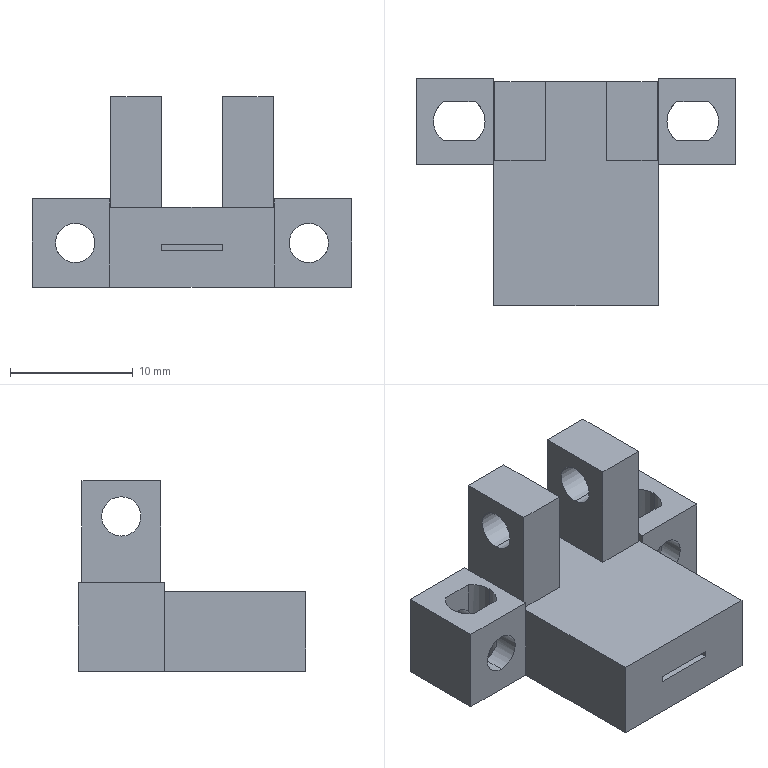Part | STEP file | 0245_027_FPML44 | 1 solid | 55 faces | box 26 x 18.5 x 15.5 mm | volume 2386 mm3 | plane 37 | cylinder 18 | commonest cylinder face diameters 3.2 x12 4 x6